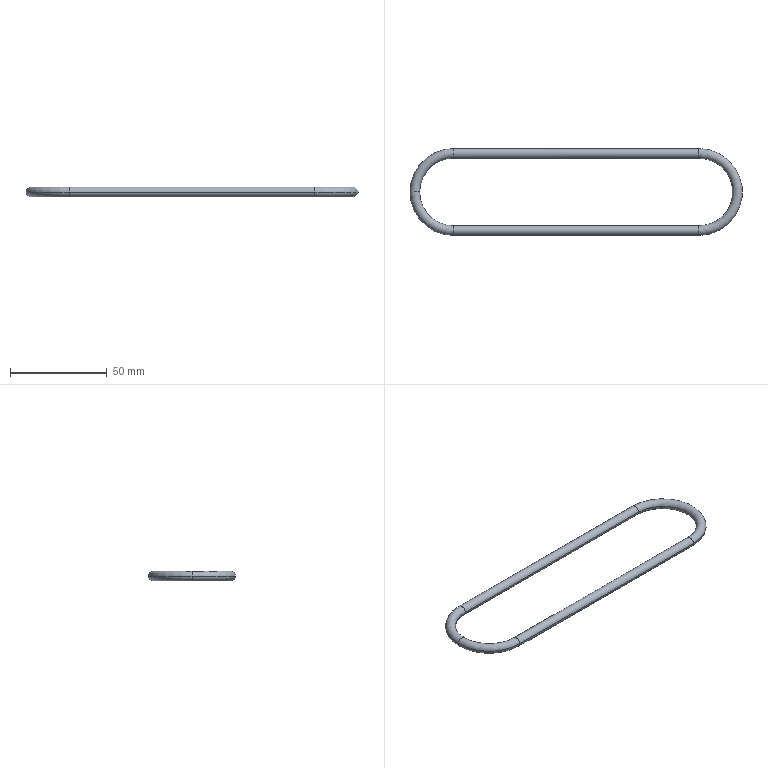Part | STEP file | MBT5-380 | 1 solid | 10 faces | box 172.168 x 45 x 5 mm | volume 7461 mm3 | torus 6 | cylinder 4 | commonest cylinder face diameters 5 x4
STEP:
#1=CARTESIAN_POINT('',(127.168,17.5,0.));
#2=VERTEX_POINT('',#1);
#3=CARTESIAN_POINT('',(127.168,22.5,0.));
#4=VERTEX_POINT('',#3);
#5=CARTESIAN_POINT('',(127.168,20.,0.));
#6=DIRECTION('',(1.,0.,0.));
#7=DIRECTION('',(0.,0.,-1.));
#8=AXIS2_PLACEMENT_3D('',#5,#6,#7);
#9=CIRCLE('',#8,2.5);
#10=EDGE_CURVE('',#2,#4,#9,.T.);
#11=ORIENTED_EDGE('',*,*,#10,.T.);
#12=CARTESIAN_POINT('',(127.168,-22.5,0.));
#13=VERTEX_POINT('',#12);
#14=CARTESIAN_POINT('',(127.168,0.,0.));
#15=DIRECTION('',(0.,0.,-1.));
#16=DIRECTION('',(-1.,0.,0.));
#17=AXIS2_PLACEMENT_3D('',#14,#15,#16);
#18=CIRCLE('',#17,22.5);
#19=EDGE_CURVE('',#4,#13,#18,.T.);
#20=ORIENTED_EDGE('',*,*,#19,.T.);
#21=CARTESIAN_POINT('',(127.168,-17.5,0.));
#22=VERTEX_POINT('',#21);
#23=CARTESIAN_POINT('',(127.168,-20.,0.));
#24=DIRECTION('',(-1.,0.,0.));
#25=DIRECTION('',(0.,0.,-1.));
#26=AXIS2_PLACEMENT_3D('',#23,#24,#25);
#27=CIRCLE('',#26,2.5);
#28=EDGE_CURVE('',#22,#13,#27,.T.);
#29=ORIENTED_EDGE('',*,*,#28,.F.);
#30=CARTESIAN_POINT('',(127.168,0.,0.));
#31=DIRECTION('',(0.,0.,-1.));
#32=DIRECTION('',(-1.,0.,0.));
#33=AXIS2_PLACEMENT_3D('',#30,#31,#32);
#34=CIRCLE('',#33,17.5);
#35=EDGE_CURVE('',#2,#22,#34,.T.);
#36=ORIENTED_EDGE('',*,*,#35,.F.);
#37=EDGE_LOOP('',(#11,#20,#29,#36));
#38=FACE_OUTER_BOUND('',#37,.T.);
#39=CARTESIAN_POINT('',(127.168,0.,0.));
#40=DIRECTION('',(0.,0.,-1.));
#41=DIRECTION('',(-1.,0.,0.));
#42=AXIS2_PLACEMENT_3D('',#39,#40,#41);
#43=TOROIDAL_SURFACE('',#42,20.,2.5);
#44=ADVANCED_FACE('',(#38),#43,.T.);
#45=CARTESIAN_POINT('',(-22.5,0.,0.));
#46=VERTEX_POINT('',#45);
#47=CARTESIAN_POINT('',(-17.5,0.,0.));
#48=VERTEX_POINT('',#47);
#49=CARTESIAN_POINT('',(-20.,0.,0.));
#50=DIRECTION('',(0.,-1.,0.));
#51=DIRECTION('',(0.,0.,-1.));
#52=AXIS2_PLACEMENT_3D('',#49,#50,#51);
#53=CIRCLE('',#52,2.5);
#54=EDGE_CURVE('',#46,#48,#53,.T.);
#55=ORIENTED_EDGE('',*,*,#54,.F.);
#56=CARTESIAN_POINT('',(0.,22.5,0.));
#57=VERTEX_POINT('',#56);
#58=CARTESIAN_POINT('',(0.,0.,0.));
#59=DIRECTION('',(0.,0.,-1.));
#60=DIRECTION('',(-1.,0.,0.));
#61=AXIS2_PLACEMENT_3D('',#58,#59,#60);
#62=CIRCLE('',#61,22.5);
#63=EDGE_CURVE('',#46,#57,#62,.T.);
#64=ORIENTED_EDGE('',*,*,#63,.T.);
#65=CARTESIAN_POINT('',(0.,17.5,0.));
#66=VERTEX_POINT('',#65);
#67=CARTESIAN_POINT('',(0.,17.5,0.));
#68=CARTESIAN_POINT('',(0.,17.5,-0.3272));
#69=CARTESIAN_POINT('',(0.,17.565,-0.6544));
#70=CARTESIAN_POINT('',(0.,17.816,-1.259));
#71=CARTESIAN_POINT('',(0.,18.001,-1.536));
#72=CARTESIAN_POINT('',(0.,18.464,-1.999));
#73=CARTESIAN_POINT('',(0.,18.741,-2.184));
#74=CARTESIAN_POINT('',(0.,19.346,-2.435));
#75=CARTESIAN_POINT('',(0.,19.673,-2.5));
#76=CARTESIAN_POINT('',(0.,20.327,-2.5));
#77=CARTESIAN_POINT('',(0.,20.654,-2.435));
#78=CARTESIAN_POINT('',(0.,21.259,-2.184));
#79=CARTESIAN_POINT('',(0.,21.536,-1.999));
#80=CARTESIAN_POINT('',(0.,21.999,-1.536));
#81=CARTESIAN_POINT('',(0.,22.184,-1.259));
#82=CARTESIAN_POINT('',(0.,22.435,-0.6544));
#83=CARTESIAN_POINT('',(0.,22.5,-0.3272));
#84=CARTESIAN_POINT('',(0.,22.5,0.));
#85=B_SPLINE_CURVE_WITH_KNOTS('',3,(#67,#68,#69,#70,#71,#72,#73,#74,#75,#76,#77,#78,#79,#80,#81,#82,#83,#84),.UNSPECIFIED.,.F.,.F.,(4,2,2,2,2,2,2,2,4),(0.75,0.8125,0.875,0.9375,1.,1.062,1.125,1.188,1.25),.UNSPECIFIED.);
#86=EDGE_CURVE('',#66,#57,#85,.T.);
#87=ORIENTED_EDGE('',*,*,#86,.F.);
#88=CARTESIAN_POINT('',(0.,0.,0.));
#89=DIRECTION('',(0.,0.,-1.));
#90=DIRECTION('',(-1.,0.,0.));
#91=AXIS2_PLACEMENT_3D('',#88,#89,#90);
#92=CIRCLE('',#91,17.5);
#93=EDGE_CURVE('',#48,#66,#92,.T.);
#94=ORIENTED_EDGE('',*,*,#93,.F.);
#95=EDGE_LOOP('',(#55,#64,#87,#94));
#96=FACE_OUTER_BOUND('',#95,.T.);
#97=CARTESIAN_POINT('',(0.,0.,0.));
#98=DIRECTION('',(0.,0.,-1.));
#99=DIRECTION('',(-1.,0.,0.));
#100=AXIS2_PLACEMENT_3D('',#97,#98,#99);
#101=TOROIDAL_SURFACE('',#100,20.,2.5);
#102=ADVANCED_FACE('',(#96),#101,.T.);
#103=CARTESIAN_POINT('',(0.,-17.5,0.));
#104=VERTEX_POINT('',#103);
#105=CARTESIAN_POINT('',(0.,-22.5,0.));
#106=VERTEX_POINT('',#105);
#107=CARTESIAN_POINT('',(0.,-20.,0.));
#108=DIRECTION('',(-1.,0.,0.));
#109=DIRECTION('',(0.,0.,-1.));
#110=AXIS2_PLACEMENT_3D('',#107,#108,#109);
#111=CIRCLE('',#110,2.5);
#112=EDGE_CURVE('',#104,#106,#111,.T.);
#113=ORIENTED_EDGE('',*,*,#112,.T.);
#114=CARTESIAN_POINT('',(0.,0.,0.));
#115=DIRECTION('',(0.,0.,-1.));
#116=DIRECTION('',(-1.,0.,0.));
#117=AXIS2_PLACEMENT_3D('',#114,#115,#116);
#118=CIRCLE('',#117,22.5);
#119=EDGE_CURVE('',#106,#46,#118,.T.);
#120=ORIENTED_EDGE('',*,*,#119,.T.);
#121=ORIENTED_EDGE('',*,*,#54,.T.);
#122=CARTESIAN_POINT('',(0.,0.,0.));
#123=DIRECTION('',(0.,0.,-1.));
#124=DIRECTION('',(-1.,0.,0.));
#125=AXIS2_PLACEMENT_3D('',#122,#123,#124);
#126=CIRCLE('',#125,17.5);
#127=EDGE_CURVE('',#104,#48,#126,.T.);
#128=ORIENTED_EDGE('',*,*,#127,.F.);
#129=EDGE_LOOP('',(#113,#120,#121,#128));
#130=FACE_OUTER_BOUND('',#129,.T.);
#131=CARTESIAN_POINT('',(0.,0.,0.));
#132=DIRECTION('',(0.,0.,-1.));
#133=DIRECTION('',(-1.,0.,0.));
#134=AXIS2_PLACEMENT_3D('',#131,#132,#133);
#135=TOROIDAL_SURFACE('',#134,20.,2.5);
#136=ADVANCED_FACE('',(#130),#135,.T.);
#137=CARTESIAN_POINT('',(127.168,20.,0.));
#138=DIRECTION('',(1.,0.,0.));
#139=DIRECTION('',(0.,0.,-1.));
#140=AXIS2_PLACEMENT_3D('',#137,#138,#139);
#141=CIRCLE('',#140,2.5);
#142=EDGE_CURVE('',#4,#2,#141,.T.);
#143=ORIENTED_EDGE('',*,*,#142,.F.);
#144=CARTESIAN_POINT('',(127.168,22.5,0.));
#145=DIRECTION('',(-1.,0.,0.));
#146=VECTOR('',#145,1000.);
#147=LINE('',#144,#146);
#148=EDGE_CURVE('',#4,#57,#147,.T.);
#149=ORIENTED_EDGE('',*,*,#148,.T.);
#150=CARTESIAN_POINT('',(0.,22.5,0.));
#151=CARTESIAN_POINT('',(0.,22.5,0.3272));
#152=CARTESIAN_POINT('',(0.,22.435,0.6544));
#153=CARTESIAN_POINT('',(0.,22.184,1.259));
#154=CARTESIAN_POINT('',(0.,21.999,1.536));
#155=CARTESIAN_POINT('',(0.,21.536,1.999));
#156=CARTESIAN_POINT('',(0.,21.259,2.184));
#157=CARTESIAN_POINT('',(0.,20.654,2.435));
#158=CARTESIAN_POINT('',(0.,20.327,2.5));
#159=CARTESIAN_POINT('',(0.,19.673,2.5));
#160=CARTESIAN_POINT('',(0.,19.346,2.435));
#161=CARTESIAN_POINT('',(0.,18.741,2.184));
#162=CARTESIAN_POINT('',(0.,18.464,1.999));
#163=CARTESIAN_POINT('',(0.,18.001,1.536));
#164=CARTESIAN_POINT('',(0.,17.816,1.259));
#165=CARTESIAN_POINT('',(0.,17.565,0.6544));
#166=CARTESIAN_POINT('',(0.,17.5,0.3272));
#167=CARTESIAN_POINT('',(0.,17.5,0.));
#168=B_SPLINE_CURVE_WITH_KNOTS('',3,(#150,#151,#152,#153,#154,#155,#156,#157,#158,#159,#160,#161,#162,#163,#164,#165,#166,#167),.UNSPECIFIED.,.F.,.F.,(4,2,2,2,2,2,2,2,4),(0.25,0.3125,0.375,0.4375,0.5,0.5625,0.625,0.6875,0.75),.UNSPECIFIED.);
#169=EDGE_CURVE('',#57,#66,#168,.T.);
#170=ORIENTED_EDGE('',*,*,#169,.T.);
#171=CARTESIAN_POINT('',(127.168,17.5,0.));
#172=DIRECTION('',(-1.,0.,0.));
#173=VECTOR('',#172,1000.);
#174=LINE('',#171,#173);
#175=EDGE_CURVE('',#2,#66,#174,.T.);
#176=ORIENTED_EDGE('',*,*,#175,.F.);
#177=EDGE_LOOP('',(#143,#149,#170,#176));
#178=FACE_OUTER_BOUND('',#177,.T.);
#179=CARTESIAN_POINT('',(127.168,20.,0.));
#180=DIRECTION('',(-1.,0.,0.));
#181=DIRECTION('',(0.,-1.,0.));
#182=AXIS2_PLACEMENT_3D('',#179,#180,#181);
#183=CYLINDRICAL_SURFACE('',#182,2.5);
#184=ADVANCED_FACE('',(#178),#183,.T.);
#185=CARTESIAN_POINT('',(127.168,-20.,0.));
#186=DIRECTION('',(-1.,0.,0.));
#187=DIRECTION('',(0.,0.,-1.));
#188=AXIS2_PLACEMENT_3D('',#185,#186,#187);
#189=CIRCLE('',#188,2.5);
#190=EDGE_CURVE('',#13,#22,#189,.T.);
#191=ORIENTED_EDGE('',*,*,#190,.T.);
#192=CARTESIAN_POINT('',(127.168,-17.5,0.));
#193=DIRECTION('',(-1.,0.,0.));
#194=VECTOR('',#193,1000.);
#195=LINE('',#192,#194);
#196=EDGE_CURVE('',#22,#104,#195,.T.);
#197=ORIENTED_EDGE('',*,*,#196,.T.);
#198=CARTESIAN_POINT('',(0.,-20.,0.));
#199=DIRECTION('',(-1.,0.,0.));
#200=DIRECTION('',(0.,0.,-1.));
#201=AXIS2_PLACEMENT_3D('',#198,#199,#200);
#202=CIRCLE('',#201,2.5);
#203=EDGE_CURVE('',#106,#104,#202,.T.);
#204=ORIENTED_EDGE('',*,*,#203,.F.);
#205=CARTESIAN_POINT('',(127.168,-22.5,0.));
#206=DIRECTION('',(-1.,0.,0.));
#207=VECTOR('',#206,1000.);
#208=LINE('',#205,#207);
#209=EDGE_CURVE('',#13,#106,#208,.T.);
#210=ORIENTED_EDGE('',*,*,#209,.F.);
#211=EDGE_LOOP('',(#191,#197,#204,#210));
#212=FACE_OUTER_BOUND('',#211,.T.);
#213=CARTESIAN_POINT('',(127.168,-20.,0.));
#214=DIRECTION('',(-1.,0.,0.));
#215=DIRECTION('',(0.,-1.,0.));
#216=AXIS2_PLACEMENT_3D('',#213,#214,#215);
#217=CYLINDRICAL_SURFACE('',#216,2.5);
#218=ADVANCED_FACE('',(#212),#217,.T.);
#219=ORIENTED_EDGE('',*,*,#119,.F.);
#220=ORIENTED_EDGE('',*,*,#203,.T.);
#221=ORIENTED_EDGE('',*,*,#127,.T.);
#222=CARTESIAN_POINT('',(-20.,0.,0.));
#223=DIRECTION('',(0.,-1.,0.));
#224=DIRECTION('',(0.,0.,-1.));
#225=AXIS2_PLACEMENT_3D('',#222,#223,#224);
#226=CIRCLE('',#225,2.5);
#227=EDGE_CURVE('',#48,#46,#226,.T.);
#228=ORIENTED_EDGE('',*,*,#227,.T.);
#229=EDGE_LOOP('',(#219,#220,#221,#228));
#230=FACE_OUTER_BOUND('',#229,.T.);
#231=CARTESIAN_POINT('',(0.,0.,0.));
#232=DIRECTION('',(0.,0.,-1.));
#233=DIRECTION('',(-1.,0.,0.));
#234=AXIS2_PLACEMENT_3D('',#231,#232,#233);
#235=TOROIDAL_SURFACE('',#234,20.,2.5);
#236=ADVANCED_FACE('',(#230),#235,.T.);
#237=ORIENTED_EDGE('',*,*,#63,.F.);
#238=ORIENTED_EDGE('',*,*,#227,.F.);
#239=ORIENTED_EDGE('',*,*,#93,.T.);
#240=ORIENTED_EDGE('',*,*,#169,.F.);
#241=EDGE_LOOP('',(#237,#238,#239,#240));
#242=FACE_OUTER_BOUND('',#241,.T.);
#243=CARTESIAN_POINT('',(0.,0.,0.));
#244=DIRECTION('',(0.,0.,-1.));
#245=DIRECTION('',(-1.,0.,0.));
#246=AXIS2_PLACEMENT_3D('',#243,#244,#245);
#247=TOROIDAL_SURFACE('',#246,20.,2.5);
#248=ADVANCED_FACE('',(#242),#247,.T.);
#249=ORIENTED_EDGE('',*,*,#196,.F.);
#250=ORIENTED_EDGE('',*,*,#28,.T.);
#251=ORIENTED_EDGE('',*,*,#209,.T.);
#252=ORIENTED_EDGE('',*,*,#112,.F.);
#253=EDGE_LOOP('',(#249,#250,#251,#252));
#254=FACE_OUTER_BOUND('',#253,.T.);
#255=CARTESIAN_POINT('',(127.168,-20.,0.));
#256=DIRECTION('',(-1.,0.,0.));
#257=DIRECTION('',(0.,-1.,0.));
#258=AXIS2_PLACEMENT_3D('',#255,#256,#257);
#259=CYLINDRICAL_SURFACE('',#258,2.5);
#260=ADVANCED_FACE('',(#254),#259,.T.);
#261=ORIENTED_EDGE('',*,*,#19,.F.);
#262=ORIENTED_EDGE('',*,*,#142,.T.);
#263=ORIENTED_EDGE('',*,*,#35,.T.);
#264=ORIENTED_EDGE('',*,*,#190,.F.);
#265=EDGE_LOOP('',(#261,#262,#263,#264));
#266=FACE_OUTER_BOUND('',#265,.T.);
#267=CARTESIAN_POINT('',(127.168,0.,0.));
#268=DIRECTION('',(0.,0.,-1.));
#269=DIRECTION('',(-1.,0.,0.));
#270=AXIS2_PLACEMENT_3D('',#267,#268,#269);
#271=TOROIDAL_SURFACE('',#270,20.,2.5);
#272=ADVANCED_FACE('',(#266),#271,.T.);
#273=ORIENTED_EDGE('',*,*,#148,.F.);
#274=ORIENTED_EDGE('',*,*,#10,.F.);
#275=ORIENTED_EDGE('',*,*,#175,.T.);
#276=ORIENTED_EDGE('',*,*,#86,.T.);
#277=EDGE_LOOP('',(#273,#274,#275,#276));
#278=FACE_OUTER_BOUND('',#277,.T.);
#279=CARTESIAN_POINT('',(127.168,20.,0.));
#280=DIRECTION('',(-1.,0.,0.));
#281=DIRECTION('',(0.,-1.,0.));
#282=AXIS2_PLACEMENT_3D('',#279,#280,#281);
#283=CYLINDRICAL_SURFACE('',#282,2.5);
#284=ADVANCED_FACE('',(#278),#283,.T.);
#285=CLOSED_SHELL('',(#44,#102,#136,#184,#218,#236,#248,#260,#272,#284));
#286=MANIFOLD_SOLID_BREP('',#285);
#287=CARTESIAN_POINT('',(0.,0.,0.));
#288=DIRECTION('',(0.,0.,1.));
#289=DIRECTION('',(1.,0.,0.));
#290=AXIS2_PLACEMENT_3D('',#287,#288,#289);
#291=(LENGTH_UNIT()NAMED_UNIT(*)SI_UNIT(.MILLI.,.METRE.));
#292=UNCERTAINTY_MEASURE_WITH_UNIT(LENGTH_MEASURE(0.00001),#291,'','');
#293=(NAMED_UNIT(*)PLANE_ANGLE_UNIT()SI_UNIT($,.RADIAN.));
#294=(NAMED_UNIT(*)SI_UNIT($,.STERADIAN.)SOLID_ANGLE_UNIT());
#295=(GEOMETRIC_REPRESENTATION_CONTEXT(3)GLOBAL_UNCERTAINTY_ASSIGNED_CONTEXT((#292))GLOBAL_UNIT_ASSIGNED_CONTEXT((#291,#293,#294))REPRESENTATION_CONTEXT('',''));
#296=ADVANCED_BREP_SHAPE_REPRESENTATION('',(#286,#290),#295);